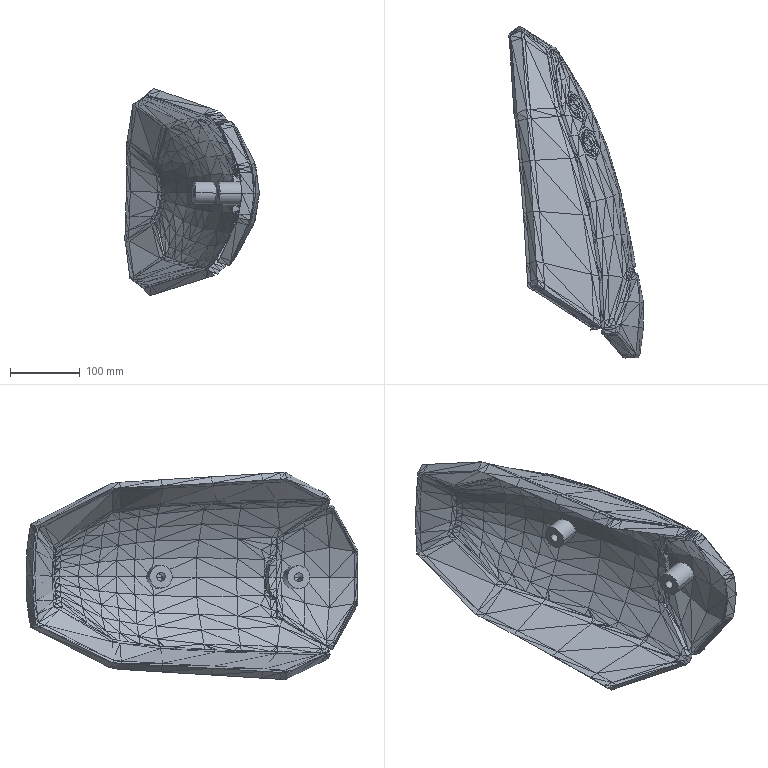Part | SolidWorks | features MirrorStock 1 | 1 solid | 1858 faces | box 192.975 x 474.444 x 296.209 mm | volume 2534423 mm3 | plane 1850 | cylinder 8 | commonest cylinder face diameters 12.5 x4 32.5 x4